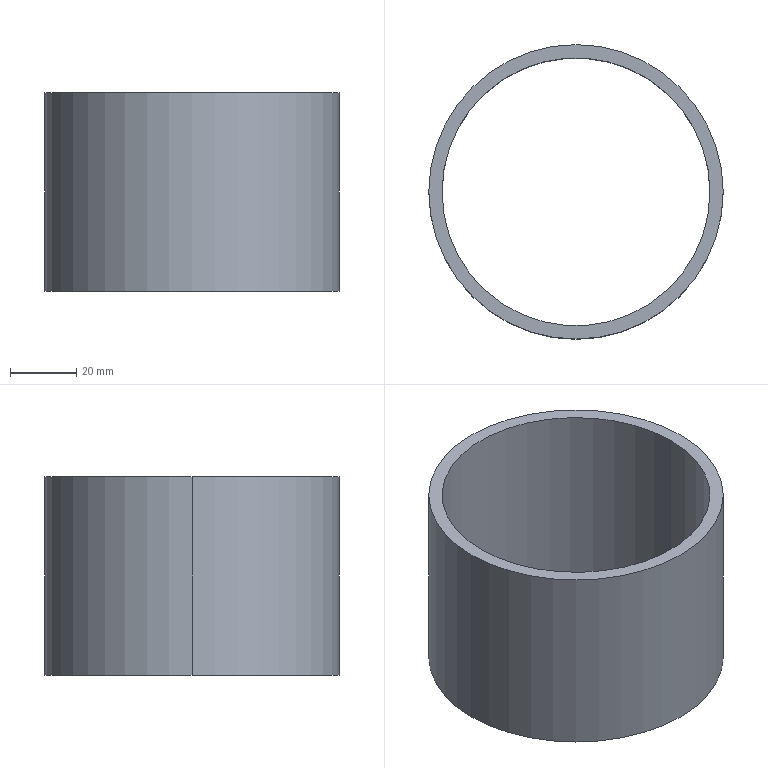Part | SolidWorks | features Extrusion 1 | 1 solid | 6 faces | box 89 x 89 x 60 mm | volume 64088 mm3 | cylinder 4 | plane 2 | commonest cylinder face diameters 81 x2 89 x2
STEP:
#1=CARTESIAN_POINT('',(-1100.5,0.,60.));
#2=VERTEX_POINT('',#1);
#3=CARTESIAN_POINT('',(-1019.5,0.,60.));
#4=VERTEX_POINT('',#3);
#5=CARTESIAN_POINT('',(-1060.,0.,60.));
#6=DIRECTION('',(0.,0.,1.));
#7=DIRECTION('',(1.,0.,0.));
#8=AXIS2_PLACEMENT_3D('',#5,#6,#7);
#9=CIRCLE('',#8,40.5);
#10=EDGE_CURVE('',#2,#4,#9,.T.);
#11=ORIENTED_EDGE('',*,*,#10,.T.);
#12=CARTESIAN_POINT('',(-1019.5,0.,0.));
#13=VERTEX_POINT('',#12);
#14=CARTESIAN_POINT('',(-1019.5,0.,60.));
#15=DIRECTION('',(0.,0.,-1.));
#16=VECTOR('',#15,1000.);
#17=LINE('',#14,#16);
#18=EDGE_CURVE('',#4,#13,#17,.T.);
#19=ORIENTED_EDGE('',*,*,#18,.T.);
#20=CARTESIAN_POINT('',(-1100.5,0.,0.));
#21=VERTEX_POINT('',#20);
#22=CARTESIAN_POINT('',(-1060.,0.,0.));
#23=DIRECTION('',(0.,0.,1.));
#24=DIRECTION('',(1.,0.,0.));
#25=AXIS2_PLACEMENT_3D('',#22,#23,#24);
#26=CIRCLE('',#25,40.5);
#27=EDGE_CURVE('',#21,#13,#26,.T.);
#28=ORIENTED_EDGE('',*,*,#27,.F.);
#29=CARTESIAN_POINT('',(-1100.5,0.,60.));
#30=DIRECTION('',(0.,0.,-1.));
#31=VECTOR('',#30,1000.);
#32=LINE('',#29,#31);
#33=EDGE_CURVE('',#2,#21,#32,.T.);
#34=ORIENTED_EDGE('',*,*,#33,.F.);
#35=EDGE_LOOP('',(#11,#19,#28,#34));
#36=FACE_OUTER_BOUND('',#35,.T.);
#37=CARTESIAN_POINT('',(-1060.,0.,60.));
#38=DIRECTION('',(0.,0.,-1.));
#39=DIRECTION('',(-1.,0.,0.));
#40=AXIS2_PLACEMENT_3D('',#37,#38,#39);
#41=CYLINDRICAL_SURFACE('',#40,40.5);
#42=ADVANCED_FACE('',(#36),#41,.F.);
#43=CARTESIAN_POINT('',(-1015.5,0.,60.));
#44=VERTEX_POINT('',#43);
#45=CARTESIAN_POINT('',(-1104.5,0.,60.));
#46=VERTEX_POINT('',#45);
#47=CARTESIAN_POINT('',(-1060.,0.,60.));
#48=DIRECTION('',(0.,0.,1.));
#49=DIRECTION('',(1.,0.,0.));
#50=AXIS2_PLACEMENT_3D('',#47,#48,#49);
#51=CIRCLE('',#50,44.5);
#52=EDGE_CURVE('',#44,#46,#51,.T.);
#53=ORIENTED_EDGE('',*,*,#52,.F.);
#54=CARTESIAN_POINT('',(-1015.5,0.,0.));
#55=VERTEX_POINT('',#54);
#56=CARTESIAN_POINT('',(-1015.5,0.,60.));
#57=DIRECTION('',(0.,0.,-1.));
#58=VECTOR('',#57,1000.);
#59=LINE('',#56,#58);
#60=EDGE_CURVE('',#44,#55,#59,.T.);
#61=ORIENTED_EDGE('',*,*,#60,.T.);
#62=CARTESIAN_POINT('',(-1104.5,0.,0.));
#63=VERTEX_POINT('',#62);
#64=CARTESIAN_POINT('',(-1060.,0.,0.));
#65=DIRECTION('',(0.,0.,1.));
#66=DIRECTION('',(1.,0.,0.));
#67=AXIS2_PLACEMENT_3D('',#64,#65,#66);
#68=CIRCLE('',#67,44.5);
#69=EDGE_CURVE('',#55,#63,#68,.T.);
#70=ORIENTED_EDGE('',*,*,#69,.T.);
#71=CARTESIAN_POINT('',(-1104.5,0.,60.));
#72=DIRECTION('',(0.,0.,-1.));
#73=VECTOR('',#72,1000.);
#74=LINE('',#71,#73);
#75=EDGE_CURVE('',#46,#63,#74,.T.);
#76=ORIENTED_EDGE('',*,*,#75,.F.);
#77=EDGE_LOOP('',(#53,#61,#70,#76));
#78=FACE_OUTER_BOUND('',#77,.T.);
#79=CARTESIAN_POINT('',(-1060.,0.,60.));
#80=DIRECTION('',(0.,0.,-1.));
#81=DIRECTION('',(-1.,0.,0.));
#82=AXIS2_PLACEMENT_3D('',#79,#80,#81);
#83=CYLINDRICAL_SURFACE('',#82,44.5);
#84=ADVANCED_FACE('',(#78),#83,.T.);
#85=CARTESIAN_POINT('',(-1060.,0.,60.));
#86=DIRECTION('',(0.,0.,1.));
#87=DIRECTION('',(1.,0.,0.));
#88=AXIS2_PLACEMENT_3D('',#85,#86,#87);
#89=CIRCLE('',#88,44.5);
#90=EDGE_CURVE('',#46,#44,#89,.T.);
#91=ORIENTED_EDGE('',*,*,#90,.T.);
#92=ORIENTED_EDGE('',*,*,#52,.T.);
#93=EDGE_LOOP('',(#91,#92));
#94=FACE_OUTER_BOUND('',#93,.T.);
#95=ORIENTED_EDGE('',*,*,#10,.F.);
#96=CARTESIAN_POINT('',(-1060.,0.,60.));
#97=DIRECTION('',(0.,0.,1.));
#98=DIRECTION('',(1.,0.,0.));
#99=AXIS2_PLACEMENT_3D('',#96,#97,#98);
#100=CIRCLE('',#99,40.5);
#101=EDGE_CURVE('',#4,#2,#100,.T.);
#102=ORIENTED_EDGE('',*,*,#101,.F.);
#103=EDGE_LOOP('',(#95,#102));
#104=FACE_BOUND('',#103,.T.);
#105=CARTESIAN_POINT('',(-1060.,0.,60.));
#106=DIRECTION('',(0.,0.,1.));
#107=DIRECTION('',(1.,0.,0.));
#108=AXIS2_PLACEMENT_3D('',#105,#106,#107);
#109=PLANE('',#108);
#110=ADVANCED_FACE('',(#94,#104),#109,.T.);
#111=CARTESIAN_POINT('',(-1060.,0.,0.));
#112=DIRECTION('',(0.,0.,1.));
#113=DIRECTION('',(1.,0.,0.));
#114=AXIS2_PLACEMENT_3D('',#111,#112,#113);
#115=CIRCLE('',#114,44.5);
#116=EDGE_CURVE('',#63,#55,#115,.T.);
#117=ORIENTED_EDGE('',*,*,#116,.F.);
#118=ORIENTED_EDGE('',*,*,#69,.F.);
#119=EDGE_LOOP('',(#117,#118));
#120=FACE_OUTER_BOUND('',#119,.T.);
#121=ORIENTED_EDGE('',*,*,#27,.T.);
#122=CARTESIAN_POINT('',(-1060.,0.,0.));
#123=DIRECTION('',(0.,0.,1.));
#124=DIRECTION('',(1.,0.,0.));
#125=AXIS2_PLACEMENT_3D('',#122,#123,#124);
#126=CIRCLE('',#125,40.5);
#127=EDGE_CURVE('',#13,#21,#126,.T.);
#128=ORIENTED_EDGE('',*,*,#127,.T.);
#129=EDGE_LOOP('',(#121,#128));
#130=FACE_BOUND('',#129,.T.);
#131=CARTESIAN_POINT('',(-1060.,0.,0.));
#132=DIRECTION('',(0.,0.,1.));
#133=DIRECTION('',(1.,0.,0.));
#134=AXIS2_PLACEMENT_3D('',#131,#132,#133);
#135=PLANE('',#134);
#136=ADVANCED_FACE('',(#120,#130),#135,.F.);
#137=ORIENTED_EDGE('',*,*,#60,.F.);
#138=ORIENTED_EDGE('',*,*,#90,.F.);
#139=ORIENTED_EDGE('',*,*,#75,.T.);
#140=ORIENTED_EDGE('',*,*,#116,.T.);
#141=EDGE_LOOP('',(#137,#138,#139,#140));
#142=FACE_OUTER_BOUND('',#141,.T.);
#143=CARTESIAN_POINT('',(-1060.,0.,60.));
#144=DIRECTION('',(0.,0.,-1.));
#145=DIRECTION('',(-1.,0.,0.));
#146=AXIS2_PLACEMENT_3D('',#143,#144,#145);
#147=CYLINDRICAL_SURFACE('',#146,44.5);
#148=ADVANCED_FACE('',(#142),#147,.T.);
#149=ORIENTED_EDGE('',*,*,#18,.F.);
#150=ORIENTED_EDGE('',*,*,#101,.T.);
#151=ORIENTED_EDGE('',*,*,#33,.T.);
#152=ORIENTED_EDGE('',*,*,#127,.F.);
#153=EDGE_LOOP('',(#149,#150,#151,#152));
#154=FACE_OUTER_BOUND('',#153,.T.);
#155=CARTESIAN_POINT('',(-1060.,0.,60.));
#156=DIRECTION('',(0.,0.,-1.));
#157=DIRECTION('',(-1.,0.,0.));
#158=AXIS2_PLACEMENT_3D('',#155,#156,#157);
#159=CYLINDRICAL_SURFACE('',#158,40.5);
#160=ADVANCED_FACE('',(#154),#159,.F.);
#161=CLOSED_SHELL('',(#42,#84,#110,#136,#148,#160));
#162=MANIFOLD_SOLID_BREP('',#161);
#163=CARTESIAN_POINT('',(0.,0.,0.));
#164=DIRECTION('',(0.,0.,1.));
#165=DIRECTION('',(1.,0.,0.));
#166=AXIS2_PLACEMENT_3D('',#163,#164,#165);
#167=(LENGTH_UNIT()NAMED_UNIT(*)SI_UNIT(.MILLI.,.METRE.));
#168=UNCERTAINTY_MEASURE_WITH_UNIT(LENGTH_MEASURE(0.00001),#167,'','');
#169=(NAMED_UNIT(*)PLANE_ANGLE_UNIT()SI_UNIT($,.RADIAN.));
#170=(NAMED_UNIT(*)SI_UNIT($,.STERADIAN.)SOLID_ANGLE_UNIT());
#171=(GEOMETRIC_REPRESENTATION_CONTEXT(3)GLOBAL_UNCERTAINTY_ASSIGNED_CONTEXT((#168))GLOBAL_UNIT_ASSIGNED_CONTEXT((#167,#169,#170))REPRESENTATION_CONTEXT('',''));
#172=ADVANCED_BREP_SHAPE_REPRESENTATION('',(#162,#166),#171);